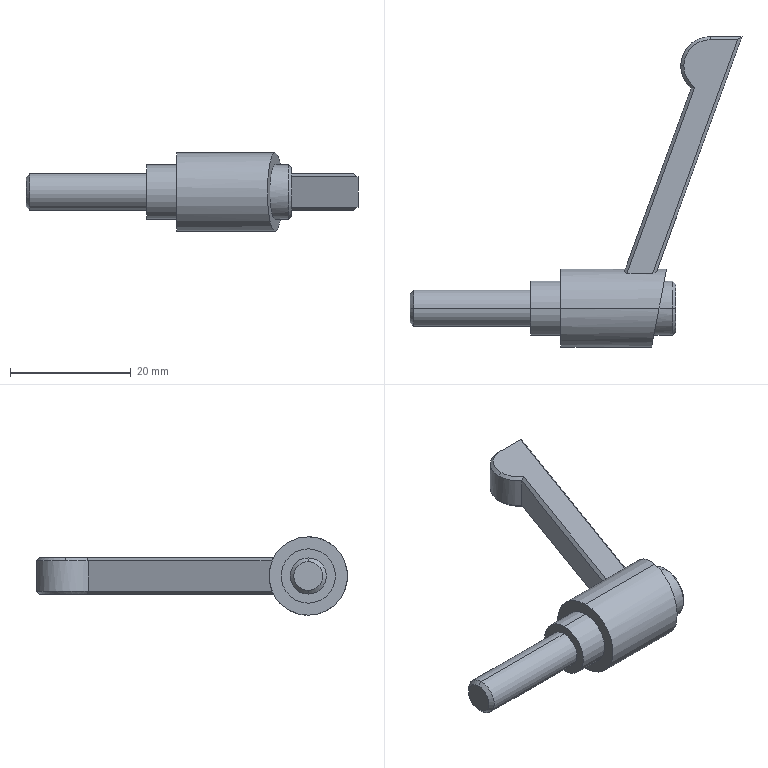Part | SolidWorks | features BaseBody 1 | 1 solid | 32 faces | box 55 x 51.5 x 13 mm | volume 4548 mm3 | plane 16 | cylinder 9 | cone 7 | commonest cylinder face diameters 9 x4 6 x2 13 x2 9.696 x1
STEP:
#1=CARTESIAN_POINT('',(15.931,5.766,-3.));
#2=VERTEX_POINT('',#1);
#3=CARTESIAN_POINT('',(20.188,5.766,-3.));
#4=VERTEX_POINT('',#3);
#5=CARTESIAN_POINT('',(25.5,5.766,-3.));
#6=DIRECTION('',(1.,0.,0.));
#7=VECTOR('',#6,1000.);
#8=LINE('',#5,#7);
#9=EDGE_CURVE('',#2,#4,#8,.T.);
#10=ORIENTED_EDGE('',*,*,#9,.T.);
#11=CARTESIAN_POINT('',(20.805,6.,-2.5));
#12=VERTEX_POINT('',#11);
#13=CARTESIAN_POINT('',(20.188,5.766,-3.));
#14=CARTESIAN_POINT('',(20.393,5.851,-2.837));
#15=CARTESIAN_POINT('',(20.599,5.929,-2.67));
#16=CARTESIAN_POINT('',(20.805,6.,-2.5));
#17=(BOUNDED_CURVE()B_SPLINE_CURVE(3,(#13,#14,#15,#16),.UNSPECIFIED.,.F.,.F.)B_SPLINE_CURVE_WITH_KNOTS((4,4),(4.562,4.647),.UNSPECIFIED.)CURVE()GEOMETRIC_REPRESENTATION_ITEM()RATIONAL_B_SPLINE_CURVE((1.,0.9994,0.9994,1.))REPRESENTATION_ITEM(''));
#18=EDGE_CURVE('',#4,#12,#17,.T.);
#19=ORIENTED_EDGE('',*,*,#18,.T.);
#20=CARTESIAN_POINT('',(20.805,6.,2.5));
#21=VERTEX_POINT('',#20);
#22=CARTESIAN_POINT('',(20.805,6.,-2.5));
#23=CARTESIAN_POINT('',(21.051,6.676,-0.8784));
#24=CARTESIAN_POINT('',(21.051,6.676,0.8784));
#25=CARTESIAN_POINT('',(20.805,6.,2.5));
#26=(BOUNDED_CURVE()B_SPLINE_CURVE(3,(#22,#23,#24,#25),.UNSPECIFIED.,.F.,.F.)B_SPLINE_CURVE_WITH_KNOTS((4,4),(5.888,6.678),.UNSPECIFIED.)CURVE()GEOMETRIC_REPRESENTATION_ITEM()RATIONAL_B_SPLINE_CURVE((1.,0.9487,0.9487,1.))REPRESENTATION_ITEM(''));
#27=EDGE_CURVE('',#12,#21,#26,.T.);
#28=ORIENTED_EDGE('',*,*,#27,.T.);
#29=CARTESIAN_POINT('',(20.188,5.766,3.));
#30=VERTEX_POINT('',#29);
#31=CARTESIAN_POINT('',(20.188,5.766,3.));
#32=CARTESIAN_POINT('',(20.393,5.851,2.837));
#33=CARTESIAN_POINT('',(20.599,5.929,2.67));
#34=CARTESIAN_POINT('',(20.805,6.,2.5));
#35=(BOUNDED_CURVE()B_SPLINE_CURVE(3,(#31,#32,#33,#34),.UNSPECIFIED.,.F.,.F.)B_SPLINE_CURVE_WITH_KNOTS((4,4),(4.562,4.647),.UNSPECIFIED.)CURVE()GEOMETRIC_REPRESENTATION_ITEM()RATIONAL_B_SPLINE_CURVE((1.,0.9994,0.9994,1.))REPRESENTATION_ITEM(''));
#36=EDGE_CURVE('',#30,#21,#35,.T.);
#37=ORIENTED_EDGE('',*,*,#36,.F.);
#38=CARTESIAN_POINT('',(15.931,5.766,3.));
#39=VERTEX_POINT('',#38);
#40=CARTESIAN_POINT('',(25.5,5.766,3.));
#41=DIRECTION('',(-1.,0.,0.));
#42=VECTOR('',#41,1000.);
#43=LINE('',#40,#42);
#44=EDGE_CURVE('',#30,#39,#43,.T.);
#45=ORIENTED_EDGE('',*,*,#44,.T.);
#46=CARTESIAN_POINT('',(15.484,6.,2.5));
#47=VERTEX_POINT('',#46);
#48=CARTESIAN_POINT('',(15.484,6.,2.5));
#49=CARTESIAN_POINT('',(15.639,5.929,2.67));
#50=CARTESIAN_POINT('',(15.788,5.851,2.837));
#51=CARTESIAN_POINT('',(15.931,5.766,3.));
#52=(BOUNDED_CURVE()B_SPLINE_CURVE(3,(#48,#49,#50,#51),.UNSPECIFIED.,.F.,.F.)B_SPLINE_CURVE_WITH_KNOTS((4,4),(5.437,5.522),.UNSPECIFIED.)CURVE()GEOMETRIC_REPRESENTATION_ITEM()RATIONAL_B_SPLINE_CURVE((1.,0.9994,0.9994,1.))REPRESENTATION_ITEM(''));
#53=EDGE_CURVE('',#47,#39,#52,.T.);
#54=ORIENTED_EDGE('',*,*,#53,.F.);
#55=CARTESIAN_POINT('',(15.484,6.,-2.5));
#56=VERTEX_POINT('',#55);
#57=CARTESIAN_POINT('',(15.484,6.,2.5));
#58=CARTESIAN_POINT('',(15.73,6.676,0.8784));
#59=CARTESIAN_POINT('',(15.73,6.676,-0.8784));
#60=CARTESIAN_POINT('',(15.484,6.,-2.5));
#61=(BOUNDED_CURVE()B_SPLINE_CURVE(3,(#57,#58,#59,#60),.UNSPECIFIED.,.F.,.F.)B_SPLINE_CURVE_WITH_KNOTS((4,4),(5.888,6.678),.UNSPECIFIED.)CURVE()GEOMETRIC_REPRESENTATION_ITEM()RATIONAL_B_SPLINE_CURVE((1.,0.9487,0.9487,1.))REPRESENTATION_ITEM(''));
#62=EDGE_CURVE('',#47,#56,#61,.T.);
#63=ORIENTED_EDGE('',*,*,#62,.T.);
#64=CARTESIAN_POINT('',(15.484,6.,-2.5));
#65=CARTESIAN_POINT('',(15.639,5.929,-2.67));
#66=CARTESIAN_POINT('',(15.788,5.851,-2.837));
#67=CARTESIAN_POINT('',(15.931,5.766,-3.));
#68=(BOUNDED_CURVE()B_SPLINE_CURVE(3,(#64,#65,#66,#67),.UNSPECIFIED.,.F.,.T.)B_SPLINE_CURVE_WITH_KNOTS((4,4),(5.437,5.522),.UNSPECIFIED.)CURVE()GEOMETRIC_REPRESENTATION_ITEM()RATIONAL_B_SPLINE_CURVE((1.,0.9994,0.9994,1.))REPRESENTATION_ITEM(''));
#69=EDGE_CURVE('',#56,#2,#68,.T.);
#70=ORIENTED_EDGE('',*,*,#69,.T.);
#71=EDGE_LOOP('',(#10,#19,#28,#37,#45,#54,#63,#70));
#72=FACE_BOUND('',#71,.T.);
#73=CARTESIAN_POINT('',(5.,0.,-6.5));
#74=VERTEX_POINT('',#73);
#75=CARTESIAN_POINT('',(5.,0.,6.5));
#76=VERTEX_POINT('',#75);
#77=CARTESIAN_POINT('',(5.,0.,0.));
#78=DIRECTION('',(1.,0.,0.));
#79=DIRECTION('',(0.,0.,-1.));
#80=AXIS2_PLACEMENT_3D('',#77,#78,#79);
#81=CIRCLE('',#80,6.5);
#82=EDGE_CURVE('',#74,#76,#81,.T.);
#83=ORIENTED_EDGE('',*,*,#82,.T.);
#84=CARTESIAN_POINT('',(21.25,0.,6.5));
#85=VERTEX_POINT('',#84);
#86=CARTESIAN_POINT('',(25.5,0.,6.5));
#87=DIRECTION('',(1.,0.,0.));
#88=VECTOR('',#87,1000.);
#89=LINE('',#86,#88);
#90=EDGE_CURVE('',#76,#85,#89,.T.);
#91=ORIENTED_EDGE('',*,*,#90,.T.);
#92=CARTESIAN_POINT('',(21.25,0.,-6.5));
#93=VERTEX_POINT('',#92);
#94=CARTESIAN_POINT('',(21.25,0.,6.5));
#95=CARTESIAN_POINT('',(23.75,13.,6.5));
#96=CARTESIAN_POINT('',(23.75,13.,-6.5));
#97=CARTESIAN_POINT('',(21.25,0.,-6.5));
#98=(BOUNDED_CURVE()B_SPLINE_CURVE(3,(#94,#95,#96,#97),.UNSPECIFIED.,.F.,.F.)B_SPLINE_CURVE_WITH_KNOTS((4,4),(4.712,7.854),.UNSPECIFIED.)CURVE()GEOMETRIC_REPRESENTATION_ITEM()RATIONAL_B_SPLINE_CURVE((1.,0.3333,0.3333,1.))REPRESENTATION_ITEM(''));
#99=EDGE_CURVE('',#85,#93,#98,.T.);
#100=ORIENTED_EDGE('',*,*,#99,.T.);
#101=CARTESIAN_POINT('',(25.5,0.,-6.5));
#102=DIRECTION('',(1.,0.,0.));
#103=VECTOR('',#102,1000.);
#104=LINE('',#101,#103);
#105=EDGE_CURVE('',#74,#93,#104,.T.);
#106=ORIENTED_EDGE('',*,*,#105,.F.);
#107=EDGE_LOOP('',(#83,#91,#100,#106));
#108=FACE_OUTER_BOUND('',#107,.T.);
#109=CARTESIAN_POINT('',(25.5,0.,0.));
#110=DIRECTION('',(1.,0.,0.));
#111=DIRECTION('',(0.,0.,-1.));
#112=AXIS2_PLACEMENT_3D('',#109,#110,#111);
#113=CYLINDRICAL_SURFACE('',#112,6.5);
#114=ADVANCED_FACE('',(#72,#108),#113,.T.);
#115=CARTESIAN_POINT('',(21.25,0.,4.5));
#116=VERTEX_POINT('',#115);
#117=CARTESIAN_POINT('',(21.25,0.,-4.5));
#118=VERTEX_POINT('',#117);
#119=CARTESIAN_POINT('',(21.25,0.,4.5));
#120=CARTESIAN_POINT('',(22.981,9.,4.5));
#121=CARTESIAN_POINT('',(22.981,9.,-4.5));
#122=CARTESIAN_POINT('',(21.25,0.,-4.5));
#123=(BOUNDED_CURVE()B_SPLINE_CURVE(3,(#119,#120,#121,#122),.UNSPECIFIED.,.F.,.F.)B_SPLINE_CURVE_WITH_KNOTS((4,4),(4.712,7.854),.UNSPECIFIED.)CURVE()GEOMETRIC_REPRESENTATION_ITEM()RATIONAL_B_SPLINE_CURVE((1.,0.3333,0.3333,1.))REPRESENTATION_ITEM(''));
#124=EDGE_CURVE('',#116,#118,#123,.T.);
#125=ORIENTED_EDGE('',*,*,#124,.F.);
#126=CARTESIAN_POINT('',(23.5,0.,4.5));
#127=VERTEX_POINT('',#126);
#128=CARTESIAN_POINT('',(24.,0.,4.5));
#129=DIRECTION('',(1.,0.,0.));
#130=VECTOR('',#129,1000.);
#131=LINE('',#128,#130);
#132=EDGE_CURVE('',#116,#127,#131,.T.);
#133=ORIENTED_EDGE('',*,*,#132,.T.);
#134=CARTESIAN_POINT('',(23.5,0.,-4.5));
#135=VERTEX_POINT('',#134);
#136=CARTESIAN_POINT('',(23.5,0.,0.));
#137=DIRECTION('',(-1.,0.,0.));
#138=DIRECTION('',(0.,0.,-1.));
#139=AXIS2_PLACEMENT_3D('',#136,#137,#138);
#140=CIRCLE('',#139,4.5);
#141=EDGE_CURVE('',#127,#135,#140,.T.);
#142=ORIENTED_EDGE('',*,*,#141,.T.);
#143=CARTESIAN_POINT('',(24.,0.,-4.5));
#144=DIRECTION('',(1.,0.,0.));
#145=VECTOR('',#144,1000.);
#146=LINE('',#143,#145);
#147=EDGE_CURVE('',#118,#135,#146,.T.);
#148=ORIENTED_EDGE('',*,*,#147,.F.);
#149=EDGE_LOOP('',(#125,#133,#142,#148));
#150=FACE_OUTER_BOUND('',#149,.T.);
#151=CARTESIAN_POINT('',(24.,0.,0.));
#152=DIRECTION('',(1.,0.,0.));
#153=DIRECTION('',(0.,0.,-1.));
#154=AXIS2_PLACEMENT_3D('',#151,#152,#153);
#155=CYLINDRICAL_SURFACE('',#154,4.5);
#156=ADVANCED_FACE('',(#150),#155,.T.);
#157=CARTESIAN_POINT('',(25.364,40.152,3.));
#158=VERTEX_POINT('',#157);
#159=CARTESIAN_POINT('',(27.164,36.629,3.));
#160=VERTEX_POINT('',#159);
#161=CARTESIAN_POINT('',(29.712,40.152,3.));
#162=DIRECTION('',(0.,0.,1.));
#163=DIRECTION('',(-1.,0.,0.));
#164=AXIS2_PLACEMENT_3D('',#161,#162,#163);
#165=CIRCLE('',#164,4.348);
#166=EDGE_CURVE('',#158,#160,#165,.T.);
#167=ORIENTED_EDGE('',*,*,#166,.F.);
#168=CARTESIAN_POINT('',(24.864,40.152,2.5));
#169=VERTEX_POINT('',#168);
#170=CARTESIAN_POINT('',(24.864,40.152,2.5));
#171=DIRECTION('',(-0.7071,0.,-0.7071));
#172=VECTOR('',#171,1000.);
#173=LINE('',#170,#172);
#174=EDGE_CURVE('',#158,#169,#173,.T.);
#175=ORIENTED_EDGE('',*,*,#174,.T.);
#176=CARTESIAN_POINT('',(26.571,36.46,2.5));
#177=VERTEX_POINT('',#176);
#178=CARTESIAN_POINT('',(29.712,40.152,2.5));
#179=DIRECTION('',(0.,0.,-1.));
#180=DIRECTION('',(1.,0.,0.));
#181=AXIS2_PLACEMENT_3D('',#178,#179,#180);
#182=CIRCLE('',#181,4.848);
#183=EDGE_CURVE('',#177,#169,#182,.T.);
#184=ORIENTED_EDGE('',*,*,#183,.F.);
#185=CARTESIAN_POINT('',(27.164,36.629,3.));
#186=CARTESIAN_POINT('',(26.966,36.568,2.835));
#187=CARTESIAN_POINT('',(26.769,36.512,2.668));
#188=CARTESIAN_POINT('',(26.571,36.46,2.5));
#189=B_SPLINE_CURVE_WITH_KNOTS('',3,(#185,#186,#187,#188),.UNSPECIFIED.,.F.,.F.,(4,4),(0.,0.0007944),.UNSPECIFIED.);
#190=EDGE_CURVE('',#160,#177,#189,.T.);
#191=ORIENTED_EDGE('',*,*,#190,.F.);
#192=EDGE_LOOP('',(#167,#175,#184,#191));
#193=FACE_OUTER_BOUND('',#192,.T.);
#194=CARTESIAN_POINT('',(29.712,40.152,2.5));
#195=DIRECTION('',(0.,0.,-1.));
#196=DIRECTION('',(-1.,0.,0.));
#197=AXIS2_PLACEMENT_3D('',#194,#195,#196);
#198=CONICAL_SURFACE('',#197,4.848,0.7854);
#199=ADVANCED_FACE('',(#193),#198,.T.);
#200=CARTESIAN_POINT('',(0.,0.,-4.5));
#201=VERTEX_POINT('',#200);
#202=CARTESIAN_POINT('',(0.,0.,4.5));
#203=VERTEX_POINT('',#202);
#204=CARTESIAN_POINT('',(0.,0.,0.));
#205=DIRECTION('',(1.,0.,0.));
#206=DIRECTION('',(0.,0.,-1.));
#207=AXIS2_PLACEMENT_3D('',#204,#205,#206);
#208=CIRCLE('',#207,4.5);
#209=EDGE_CURVE('',#201,#203,#208,.T.);
#210=ORIENTED_EDGE('',*,*,#209,.T.);
#211=CARTESIAN_POINT('',(5.,0.,4.5));
#212=VERTEX_POINT('',#211);
#213=CARTESIAN_POINT('',(24.,0.,4.5));
#214=DIRECTION('',(1.,0.,0.));
#215=VECTOR('',#214,1000.);
#216=LINE('',#213,#215);
#217=EDGE_CURVE('',#203,#212,#216,.T.);
#218=ORIENTED_EDGE('',*,*,#217,.T.);
#219=CARTESIAN_POINT('',(5.,0.,-4.5));
#220=VERTEX_POINT('',#219);
#221=CARTESIAN_POINT('',(5.,0.,0.));
#222=DIRECTION('',(1.,0.,0.));
#223=DIRECTION('',(0.,0.,-1.));
#224=AXIS2_PLACEMENT_3D('',#221,#222,#223);
#225=CIRCLE('',#224,4.5);
#226=EDGE_CURVE('',#220,#212,#225,.T.);
#227=ORIENTED_EDGE('',*,*,#226,.F.);
#228=CARTESIAN_POINT('',(24.,0.,-4.5));
#229=DIRECTION('',(1.,0.,0.));
#230=VECTOR('',#229,1000.);
#231=LINE('',#228,#230);
#232=EDGE_CURVE('',#201,#220,#231,.T.);
#233=ORIENTED_EDGE('',*,*,#232,.F.);
#234=EDGE_LOOP('',(#210,#218,#227,#233));
#235=FACE_OUTER_BOUND('',#234,.T.);
#236=CARTESIAN_POINT('',(24.,0.,0.));
#237=DIRECTION('',(1.,0.,0.));
#238=DIRECTION('',(0.,0.,-1.));
#239=AXIS2_PLACEMENT_3D('',#236,#237,#238);
#240=CYLINDRICAL_SURFACE('',#239,4.5);
#241=ADVANCED_FACE('',(#235),#240,.T.);
#242=CARTESIAN_POINT('',(24.,0.,4.));
#243=VERTEX_POINT('',#242);
#244=CARTESIAN_POINT('',(24.,0.,-4.));
#245=VERTEX_POINT('',#244);
#246=CARTESIAN_POINT('',(24.,0.,0.));
#247=DIRECTION('',(-1.,0.,0.));
#248=DIRECTION('',(0.,0.,1.));
#249=AXIS2_PLACEMENT_3D('',#246,#247,#248);
#250=CIRCLE('',#249,4.);
#251=EDGE_CURVE('',#243,#245,#250,.T.);
#252=ORIENTED_EDGE('',*,*,#251,.T.);
#253=CARTESIAN_POINT('',(23.5,0.,-4.5));
#254=DIRECTION('',(-0.7071,0.,-0.7071));
#255=VECTOR('',#254,1000.);
#256=LINE('',#253,#255);
#257=EDGE_CURVE('',#245,#135,#256,.T.);
#258=ORIENTED_EDGE('',*,*,#257,.T.);
#259=ORIENTED_EDGE('',*,*,#141,.F.);
#260=CARTESIAN_POINT('',(23.5,0.,4.5));
#261=DIRECTION('',(-0.7071,0.,0.7071));
#262=VECTOR('',#261,1000.);
#263=LINE('',#260,#262);
#264=EDGE_CURVE('',#243,#127,#263,.T.);
#265=ORIENTED_EDGE('',*,*,#264,.F.);
#266=EDGE_LOOP('',(#252,#258,#259,#265));
#267=FACE_OUTER_BOUND('',#266,.T.);
#268=CARTESIAN_POINT('',(23.5,0.,0.));
#269=DIRECTION('',(-1.,0.,0.));
#270=DIRECTION('',(0.,0.,1.));
#271=AXIS2_PLACEMENT_3D('',#268,#269,#270);
#272=CONICAL_SURFACE('',#271,4.5,0.7854);
#273=ADVANCED_FACE('',(#267),#272,.T.);
#274=CARTESIAN_POINT('',(0.,0.,3.));
#275=VERTEX_POINT('',#274);
#276=CARTESIAN_POINT('',(0.,0.,-3.));
#277=VERTEX_POINT('',#276);
#278=CARTESIAN_POINT('',(0.,0.,0.));
#279=DIRECTION('',(-1.,0.,0.));
#280=DIRECTION('',(0.,0.,1.));
#281=AXIS2_PLACEMENT_3D('',#278,#279,#280);
#282=CIRCLE('',#281,3.);
#283=EDGE_CURVE('',#275,#277,#282,.T.);
#284=ORIENTED_EDGE('',*,*,#283,.T.);
#285=CARTESIAN_POINT('',(-19.387,0.,-3.));
#286=VERTEX_POINT('',#285);
#287=CARTESIAN_POINT('',(0.,0.,-3.));
#288=DIRECTION('',(-1.,0.,0.));
#289=VECTOR('',#288,1000.);
#290=LINE('',#287,#289);
#291=EDGE_CURVE('',#277,#286,#290,.T.);
#292=ORIENTED_EDGE('',*,*,#291,.T.);
#293=CARTESIAN_POINT('',(-19.387,0.,3.));
#294=VERTEX_POINT('',#293);
#295=CARTESIAN_POINT('',(-19.387,0.,0.));
#296=DIRECTION('',(1.,0.,0.));
#297=DIRECTION('',(0.,0.,1.));
#298=AXIS2_PLACEMENT_3D('',#295,#296,#297);
#299=CIRCLE('',#298,3.);
#300=EDGE_CURVE('',#286,#294,#299,.T.);
#301=ORIENTED_EDGE('',*,*,#300,.T.);
#302=CARTESIAN_POINT('',(0.,0.,3.));
#303=DIRECTION('',(-1.,0.,0.));
#304=VECTOR('',#303,1000.);
#305=LINE('',#302,#304);
#306=EDGE_CURVE('',#275,#294,#305,.T.);
#307=ORIENTED_EDGE('',*,*,#306,.F.);
#308=EDGE_LOOP('',(#284,#292,#301,#307));
#309=FACE_OUTER_BOUND('',#308,.T.);
#310=CARTESIAN_POINT('',(0.,0.,0.));
#311=DIRECTION('',(-1.,0.,0.));
#312=DIRECTION('',(0.,0.,1.));
#313=AXIS2_PLACEMENT_3D('',#310,#311,#312);
#314=CYLINDRICAL_SURFACE('',#313,3.);
#315=ADVANCED_FACE('',(#309),#314,.T.);
#316=CARTESIAN_POINT('',(-20.,0.,-2.387));
#317=VERTEX_POINT('',#316);
#318=CARTESIAN_POINT('',(-20.,0.,2.387));
#319=VERTEX_POINT('',#318);
#320=CARTESIAN_POINT('',(-20.,0.,0.));
#321=DIRECTION('',(1.,0.,0.));
#322=DIRECTION('',(0.,0.,-1.));
#323=AXIS2_PLACEMENT_3D('',#320,#321,#322);
#324=CIRCLE('',#323,2.387);
#325=EDGE_CURVE('',#317,#319,#324,.T.);
#326=ORIENTED_EDGE('',*,*,#325,.T.);
#327=CARTESIAN_POINT('',(-19.386,0.,3.));
#328=DIRECTION('',(0.7071,0.,0.7071));
#329=VECTOR('',#328,1000.);
#330=LINE('',#327,#329);
#331=EDGE_CURVE('',#319,#294,#330,.T.);
#332=ORIENTED_EDGE('',*,*,#331,.T.);
#333=ORIENTED_EDGE('',*,*,#300,.F.);
#334=CARTESIAN_POINT('',(-19.386,0.,-3.));
#335=DIRECTION('',(0.7071,0.,-0.7071));
#336=VECTOR('',#335,1000.);
#337=LINE('',#334,#336);
#338=EDGE_CURVE('',#317,#286,#337,.T.);
#339=ORIENTED_EDGE('',*,*,#338,.F.);
#340=EDGE_LOOP('',(#326,#332,#333,#339));
#341=FACE_OUTER_BOUND('',#340,.T.);
#342=CARTESIAN_POINT('',(-19.386,0.,0.));
#343=DIRECTION('',(1.,0.,0.));
#344=DIRECTION('',(0.,0.,-1.));
#345=AXIS2_PLACEMENT_3D('',#342,#343,#344);
#346=CONICAL_SURFACE('',#345,3.,0.7854);
#347=ADVANCED_FACE('',(#341),#346,.T.);
#348=ORIENTED_EDGE('',*,*,#90,.F.);
#349=CARTESIAN_POINT('',(5.,0.,0.));
#350=DIRECTION('',(1.,0.,0.));
#351=DIRECTION('',(0.,0.,-1.));
#352=AXIS2_PLACEMENT_3D('',#349,#350,#351);
#353=CIRCLE('',#352,6.5);
#354=EDGE_CURVE('',#76,#74,#353,.T.);
#355=ORIENTED_EDGE('',*,*,#354,.T.);
#356=ORIENTED_EDGE('',*,*,#105,.T.);
#357=CARTESIAN_POINT('',(21.25,0.,-6.5));
#358=CARTESIAN_POINT('',(18.75,-13.,-6.5));
#359=CARTESIAN_POINT('',(18.75,-13.,6.5));
#360=CARTESIAN_POINT('',(21.25,0.,6.5));
#361=(BOUNDED_CURVE()B_SPLINE_CURVE(3,(#357,#358,#359,#360),.UNSPECIFIED.,.F.,.F.)B_SPLINE_CURVE_WITH_KNOTS((4,4),(1.571,4.712),.UNSPECIFIED.)CURVE()GEOMETRIC_REPRESENTATION_ITEM()RATIONAL_B_SPLINE_CURVE((1.,0.3333,0.3333,1.))REPRESENTATION_ITEM(''));
#362=EDGE_CURVE('',#93,#85,#361,.T.);
#363=ORIENTED_EDGE('',*,*,#362,.T.);
#364=EDGE_LOOP('',(#348,#355,#356,#363));
#365=FACE_OUTER_BOUND('',#364,.T.);
#366=CARTESIAN_POINT('',(25.5,0.,0.));
#367=DIRECTION('',(1.,0.,0.));
#368=DIRECTION('',(0.,0.,-1.));
#369=AXIS2_PLACEMENT_3D('',#366,#367,#368);
#370=CYLINDRICAL_SURFACE('',#369,6.5);
#371=ADVANCED_FACE('',(#365),#370,.T.);
#372=ORIENTED_EDGE('',*,*,#362,.F.);
#373=ORIENTED_EDGE('',*,*,#99,.F.);
#374=EDGE_LOOP('',(#372,#373));
#375=FACE_OUTER_BOUND('',#374,.T.);
#376=CARTESIAN_POINT('',(21.25,0.,-4.5));
#377=CARTESIAN_POINT('',(19.519,-9.,-4.5));
#378=CARTESIAN_POINT('',(19.519,-9.,4.5));
#379=CARTESIAN_POINT('',(21.25,0.,4.5));
#380=(BOUNDED_CURVE()B_SPLINE_CURVE(3,(#376,#377,#378,#379),.UNSPECIFIED.,.F.,.F.)B_SPLINE_CURVE_WITH_KNOTS((4,4),(1.571,4.712),.UNSPECIFIED.)CURVE()GEOMETRIC_REPRESENTATION_ITEM()RATIONAL_B_SPLINE_CURVE((1.,0.3333,0.3333,1.))REPRESENTATION_ITEM(''));
#381=EDGE_CURVE('',#118,#116,#380,.T.);
#382=ORIENTED_EDGE('',*,*,#381,.T.);
#383=ORIENTED_EDGE('',*,*,#124,.T.);
#384=EDGE_LOOP('',(#382,#383));
#385=FACE_BOUND('',#384,.T.);
#386=CARTESIAN_POINT('',(22.5,6.5,6.5));
#387=DIRECTION('',(0.982,-0.1888,0.));
#388=DIRECTION('',(0.1888,0.982,0.));
#389=AXIS2_PLACEMENT_3D('',#386,#387,#388);
#390=PLANE('',#389);
#391=ADVANCED_FACE('',(#375,#385),#390,.T.);
#392=CARTESIAN_POINT('',(34.286,44.5,-3.));
#393=VERTEX_POINT('',#392);
#394=CARTESIAN_POINT('',(20.188,5.766,-3.));
#395=DIRECTION('',(0.342,0.9397,0.));
#396=VECTOR('',#395,1000.);
#397=LINE('',#394,#396);
#398=EDGE_CURVE('',#4,#393,#397,.T.);
#399=ORIENTED_EDGE('',*,*,#398,.F.);
#400=ORIENTED_EDGE('',*,*,#9,.F.);
#401=CARTESIAN_POINT('',(27.164,36.629,-3.));
#402=VERTEX_POINT('',#401);
#403=CARTESIAN_POINT('',(27.164,36.629,-3.));
#404=DIRECTION('',(-0.342,-0.9397,0.));
#405=VECTOR('',#404,1000.);
#406=LINE('',#403,#405);
#407=EDGE_CURVE('',#402,#2,#406,.T.);
#408=ORIENTED_EDGE('',*,*,#407,.F.);
#409=CARTESIAN_POINT('',(29.744,44.5,-3.));
#410=VERTEX_POINT('',#409);
#411=CARTESIAN_POINT('',(29.712,40.152,-3.));
#412=DIRECTION('',(0.,0.,1.));
#413=DIRECTION('',(1.,0.,0.));
#414=AXIS2_PLACEMENT_3D('',#411,#412,#413);
#415=CIRCLE('',#414,4.348);
#416=EDGE_CURVE('',#410,#402,#415,.T.);
#417=ORIENTED_EDGE('',*,*,#416,.F.);
#418=CARTESIAN_POINT('',(29.712,44.5,-3.));
#419=DIRECTION('',(-1.,0.,0.));
#420=VECTOR('',#419,1000.);
#421=LINE('',#418,#420);
#422=EDGE_CURVE('',#393,#410,#421,.T.);
#423=ORIENTED_EDGE('',*,*,#422,.F.);
#424=EDGE_LOOP('',(#399,#400,#408,#417,#423));
#425=FACE_OUTER_BOUND('',#424,.T.);
#426=CARTESIAN_POINT('',(29.712,40.152,-3.));
#427=DIRECTION('',(0.,0.,1.));
#428=DIRECTION('',(1.,0.,0.));
#429=AXIS2_PLACEMENT_3D('',#426,#427,#428);
#430=PLANE('',#429);
#431=ADVANCED_FACE('',(#425),#430,.F.);
#432=CARTESIAN_POINT('',(26.571,36.46,2.5));
#433=DIRECTION('',(-0.342,-0.9397,0.));
#434=VECTOR('',#433,1000.);
#435=LINE('',#432,#434);
#436=EDGE_CURVE('',#177,#47,#435,.T.);
#437=ORIENTED_EDGE('',*,*,#436,.F.);
#438=CARTESIAN_POINT('',(26.571,36.46,-2.5));
#439=VERTEX_POINT('',#438);
#440=CARTESIAN_POINT('',(26.571,36.46,3.));
#441=DIRECTION('',(0.,0.,1.));
#442=VECTOR('',#441,1000.);
#443=LINE('',#440,#442);
#444=EDGE_CURVE('',#439,#177,#443,.T.);
#445=ORIENTED_EDGE('',*,*,#444,.F.);
#446=CARTESIAN_POINT('',(26.571,36.46,-2.5));
#447=DIRECTION('',(0.342,0.9397,0.));
#448=VECTOR('',#447,1000.);
#449=LINE('',#446,#448);
#450=EDGE_CURVE('',#56,#439,#449,.T.);
#451=ORIENTED_EDGE('',*,*,#450,.F.);
#452=ORIENTED_EDGE('',*,*,#62,.F.);
#453=EDGE_LOOP('',(#437,#445,#451,#452));
#454=FACE_OUTER_BOUND('',#453,.T.);
#455=CARTESIAN_POINT('',(26.571,36.46,3.));
#456=DIRECTION('',(0.9397,-0.342,0.));
#457=DIRECTION('',(0.342,0.9397,0.));
#458=AXIS2_PLACEMENT_3D('',#455,#456,#457);
#459=PLANE('',#458);
#460=ADVANCED_FACE('',(#454),#459,.F.);
#461=CARTESIAN_POINT('',(34.286,44.5,3.));
#462=VERTEX_POINT('',#461);
#463=CARTESIAN_POINT('',(20.188,5.766,3.));
#464=DIRECTION('',(0.342,0.9397,0.));
#465=VECTOR('',#464,1000.);
#466=LINE('',#463,#465);
#467=EDGE_CURVE('',#30,#462,#466,.T.);
#468=ORIENTED_EDGE('',*,*,#467,.T.);
#469=CARTESIAN_POINT('',(29.744,44.5,3.));
#470=VERTEX_POINT('',#469);
#471=CARTESIAN_POINT('',(29.712,44.5,3.));
#472=DIRECTION('',(-1.,0.,0.));
#473=VECTOR('',#472,1000.);
#474=LINE('',#471,#473);
#475=EDGE_CURVE('',#462,#470,#474,.T.);
#476=ORIENTED_EDGE('',*,*,#475,.T.);
#477=CARTESIAN_POINT('',(29.712,40.152,3.));
#478=DIRECTION('',(0.,0.,1.));
#479=DIRECTION('',(-1.,0.,0.));
#480=AXIS2_PLACEMENT_3D('',#477,#478,#479);
#481=CIRCLE('',#480,4.348);
#482=EDGE_CURVE('',#470,#158,#481,.T.);
#483=ORIENTED_EDGE('',*,*,#482,.T.);
#484=ORIENTED_EDGE('',*,*,#166,.T.);
#485=CARTESIAN_POINT('',(27.164,36.629,3.));
#486=DIRECTION('',(-0.342,-0.9397,0.));
#487=VECTOR('',#486,1000.);
#488=LINE('',#485,#487);
#489=EDGE_CURVE('',#160,#39,#488,.T.);
#490=ORIENTED_EDGE('',*,*,#489,.T.);
#491=ORIENTED_EDGE('',*,*,#44,.F.);
#492=EDGE_LOOP('',(#468,#476,#483,#484,#490,#491));
#493=FACE_OUTER_BOUND('',#492,.T.);
#494=CARTESIAN_POINT('',(29.712,40.152,3.));
#495=DIRECTION('',(0.,0.,1.));
#496=DIRECTION('',(1.,0.,0.));
#497=AXIS2_PLACEMENT_3D('',#494,#495,#496);
#498=PLANE('',#497);
#499=ADVANCED_FACE('',(#493),#498,.T.);
#500=CARTESIAN_POINT('',(35.,45.,-2.5));
#501=VERTEX_POINT('',#500);
#502=CARTESIAN_POINT('',(18.621,0.,-2.5));
#503=DIRECTION('',(-0.342,-0.9397,0.));
#504=VECTOR('',#503,1000.);
#505=LINE('',#502,#504);
#506=EDGE_CURVE('',#501,#12,#505,.T.);
#507=ORIENTED_EDGE('',*,*,#506,.F.);
#508=CARTESIAN_POINT('',(35.,45.,2.5));
#509=VERTEX_POINT('',#508);
#510=CARTESIAN_POINT('',(35.,45.,3.));
#511=DIRECTION('',(0.,0.,-1.));
#512=VECTOR('',#511,1000.);
#513=LINE('',#510,#512);
#514=EDGE_CURVE('',#509,#501,#513,.T.);
#515=ORIENTED_EDGE('',*,*,#514,.F.);
#516=CARTESIAN_POINT('',(18.621,0.,2.5));
#517=DIRECTION('',(0.342,0.9397,0.));
#518=VECTOR('',#517,1000.);
#519=LINE('',#516,#518);
#520=EDGE_CURVE('',#21,#509,#519,.T.);
#521=ORIENTED_EDGE('',*,*,#520,.F.);
#522=ORIENTED_EDGE('',*,*,#27,.F.);
#523=EDGE_LOOP('',(#507,#515,#521,#522));
#524=FACE_OUTER_BOUND('',#523,.T.);
#525=CARTESIAN_POINT('',(18.621,0.,3.));
#526=DIRECTION('',(-0.9397,0.342,0.));
#527=DIRECTION('',(-0.342,-0.9397,0.));
#528=AXIS2_PLACEMENT_3D('',#525,#526,#527);
#529=PLANE('',#528);
#530=ADVANCED_FACE('',(#524),#529,.F.);
#531=ORIENTED_EDGE('',*,*,#82,.F.);
#532=ORIENTED_EDGE('',*,*,#354,.F.);
#533=EDGE_LOOP('',(#531,#532));
#534=FACE_OUTER_BOUND('',#533,.T.);
#535=ORIENTED_EDGE('',*,*,#226,.T.);
#536=CARTESIAN_POINT('',(5.,0.,0.));
#537=DIRECTION('',(1.,0.,0.));
#538=DIRECTION('',(0.,0.,-1.));
#539=AXIS2_PLACEMENT_3D('',#536,#537,#538);
#540=CIRCLE('',#539,4.5);
#541=EDGE_CURVE('',#212,#220,#540,.T.);
#542=ORIENTED_EDGE('',*,*,#541,.T.);
#543=EDGE_LOOP('',(#535,#542));
#544=FACE_BOUND('',#543,.T.);
#545=CARTESIAN_POINT('',(5.,-6.5,6.5));
#546=DIRECTION('',(-1.,0.,0.));
#547=DIRECTION('',(0.,0.,1.));
#548=AXIS2_PLACEMENT_3D('',#545,#546,#547);
#549=PLANE('',#548);
#550=ADVANCED_FACE('',(#534,#544),#549,.T.);
#551=ORIENTED_EDGE('',*,*,#132,.F.);
#552=ORIENTED_EDGE('',*,*,#381,.F.);
#553=ORIENTED_EDGE('',*,*,#147,.T.);
#554=CARTESIAN_POINT('',(23.5,0.,0.));
#555=DIRECTION('',(-1.,0.,0.));
#556=DIRECTION('',(0.,0.,-1.));
#557=AXIS2_PLACEMENT_3D('',#554,#555,#556);
#558=CIRCLE('',#557,4.5);
#559=EDGE_CURVE('',#135,#127,#558,.T.);
#560=ORIENTED_EDGE('',*,*,#559,.T.);
#561=EDGE_LOOP('',(#551,#552,#553,#560));
#562=FACE_OUTER_BOUND('',#561,.T.);
#563=CARTESIAN_POINT('',(24.,0.,0.));
#564=DIRECTION('',(1.,0.,0.));
#565=DIRECTION('',(0.,0.,-1.));
#566=AXIS2_PLACEMENT_3D('',#563,#564,#565);
#567=CYLINDRICAL_SURFACE('',#566,4.5);
#568=ADVANCED_FACE('',(#562),#567,.T.);
#569=CARTESIAN_POINT('',(29.746,45.,-2.5));
#570=VERTEX_POINT('',#569);
#571=CARTESIAN_POINT('',(35.,45.,-2.5));
#572=DIRECTION('',(-1.,0.,0.));
#573=VECTOR('',#572,1000.);
#574=LINE('',#571,#573);
#575=EDGE_CURVE('',#501,#570,#574,.T.);
#576=ORIENTED_EDGE('',*,*,#575,.F.);
#577=CARTESIAN_POINT('',(34.286,44.5,-3.));
#578=DIRECTION('',(0.7106,0.4975,0.4975));
#579=VECTOR('',#578,1000.);
#580=LINE('',#577,#579);
#581=EDGE_CURVE('',#393,#501,#580,.T.);
#582=ORIENTED_EDGE('',*,*,#581,.F.);
#583=ORIENTED_EDGE('',*,*,#422,.T.);
#584=CARTESIAN_POINT('',(29.746,45.,-2.5));
#585=CARTESIAN_POINT('',(29.745,44.833,-2.667));
#586=CARTESIAN_POINT('',(29.745,44.667,-2.833));
#587=CARTESIAN_POINT('',(29.744,44.5,-3.));
#588=B_SPLINE_CURVE_WITH_KNOTS('',3,(#584,#585,#586,#587),.UNSPECIFIED.,.F.,.F.,(4,4),(0.,1.),.UNSPECIFIED.);
#589=EDGE_CURVE('',#570,#410,#588,.T.);
#590=ORIENTED_EDGE('',*,*,#589,.F.);
#591=EDGE_LOOP('',(#576,#582,#583,#590));
#592=FACE_OUTER_BOUND('',#591,.T.);
#593=CARTESIAN_POINT('',(35.,45.,-2.5));
#594=DIRECTION('',(0.,-0.7071,0.7071));
#595=DIRECTION('',(0.,-0.7071,-0.7071));
#596=AXIS2_PLACEMENT_3D('',#593,#594,#595);
#597=PLANE('',#596);
#598=ADVANCED_FACE('',(#592),#597,.F.);
#599=ORIENTED_EDGE('',*,*,#398,.T.);
#600=ORIENTED_EDGE('',*,*,#581,.T.);
#601=ORIENTED_EDGE('',*,*,#506,.T.);
#602=ORIENTED_EDGE('',*,*,#18,.F.);
#603=EDGE_LOOP('',(#599,#600,#601,#602));
#604=FACE_OUTER_BOUND('',#603,.T.);
#605=CARTESIAN_POINT('',(18.621,0.,-2.5));
#606=DIRECTION('',(-0.6645,0.2418,0.7071));
#607=DIRECTION('',(0.7287,0.,0.6848));
#608=AXIS2_PLACEMENT_3D('',#605,#606,#607);
#609=PLANE('',#608);
#610=ADVANCED_FACE('',(#604),#609,.F.);
#611=ORIENTED_EDGE('',*,*,#450,.T.);
#612=CARTESIAN_POINT('',(27.164,36.629,-3.));
#613=CARTESIAN_POINT('',(26.966,36.568,-2.835));
#614=CARTESIAN_POINT('',(26.769,36.512,-2.668));
#615=CARTESIAN_POINT('',(26.571,36.46,-2.5));
#616=B_SPLINE_CURVE_WITH_KNOTS('',3,(#612,#613,#614,#615),.UNSPECIFIED.,.F.,.F.,(4,4),(0.,0.0007944),.UNSPECIFIED.);
#617=EDGE_CURVE('',#402,#439,#616,.T.);
#618=ORIENTED_EDGE('',*,*,#617,.F.);
#619=ORIENTED_EDGE('',*,*,#407,.T.);
#620=ORIENTED_EDGE('',*,*,#69,.F.);
#621=EDGE_LOOP('',(#611,#618,#619,#620));
#622=FACE_OUTER_BOUND('',#621,.T.);
#623=CARTESIAN_POINT('',(26.571,36.46,-2.5));
#624=DIRECTION('',(0.6645,-0.2418,0.7071));
#625=DIRECTION('',(0.7287,0.,-0.6848));
#626=AXIS2_PLACEMENT_3D('',#623,#624,#625);
#627=PLANE('',#626);
#628=ADVANCED_FACE('',(#622),#627,.F.);
#629=ORIENTED_EDGE('',*,*,#589,.T.);
#630=ORIENTED_EDGE('',*,*,#416,.T.);
#631=ORIENTED_EDGE('',*,*,#617,.T.);
#632=CARTESIAN_POINT('',(29.712,40.152,-2.5));
#633=DIRECTION('',(0.,0.,-1.));
#634=DIRECTION('',(1.,0.,0.));
#635=AXIS2_PLACEMENT_3D('',#632,#633,#634);
#636=CIRCLE('',#635,4.848);
#637=EDGE_CURVE('',#439,#570,#636,.T.);
#638=ORIENTED_EDGE('',*,*,#637,.T.);
#639=EDGE_LOOP('',(#629,#630,#631,#638));
#640=FACE_OUTER_BOUND('',#639,.T.);
#641=CARTESIAN_POINT('',(29.712,40.152,-2.5));
#642=DIRECTION('',(0.,0.,1.));
#643=DIRECTION('',(1.,0.,0.));
#644=AXIS2_PLACEMENT_3D('',#641,#642,#643);
#645=CONICAL_SURFACE('',#644,4.848,0.7854);
#646=ADVANCED_FACE('',(#640),#645,.T.);
#647=ORIENTED_EDGE('',*,*,#190,.T.);
#648=ORIENTED_EDGE('',*,*,#436,.T.);
#649=ORIENTED_EDGE('',*,*,#53,.T.);
#650=ORIENTED_EDGE('',*,*,#489,.F.);
#651=EDGE_LOOP('',(#647,#648,#649,#650));
#652=FACE_OUTER_BOUND('',#651,.T.);
#653=CARTESIAN_POINT('',(28.595,40.559,3.));
#654=DIRECTION('',(-0.6645,0.2418,0.7071));
#655=DIRECTION('',(0.7287,0.,0.6848));
#656=AXIS2_PLACEMENT_3D('',#653,#654,#655);
#657=PLANE('',#656);
#658=ADVANCED_FACE('',(#652),#657,.T.);
#659=CARTESIAN_POINT('',(29.746,45.,2.5));
#660=VERTEX_POINT('',#659);
#661=CARTESIAN_POINT('',(29.746,45.,3.));
#662=DIRECTION('',(0.,0.,-1.));
#663=VECTOR('',#662,1000.);
#664=LINE('',#661,#663);
#665=EDGE_CURVE('',#660,#570,#664,.T.);
#666=ORIENTED_EDGE('',*,*,#665,.T.);
#667=ORIENTED_EDGE('',*,*,#637,.F.);
#668=ORIENTED_EDGE('',*,*,#444,.T.);
#669=ORIENTED_EDGE('',*,*,#183,.T.);
#670=CARTESIAN_POINT('',(29.712,40.152,2.5));
#671=DIRECTION('',(0.,0.,-1.));
#672=DIRECTION('',(1.,0.,0.));
#673=AXIS2_PLACEMENT_3D('',#670,#671,#672);
#674=CIRCLE('',#673,4.848);
#675=EDGE_CURVE('',#169,#660,#674,.T.);
#676=ORIENTED_EDGE('',*,*,#675,.T.);
#677=EDGE_LOOP('',(#666,#667,#668,#669,#676));
#678=FACE_OUTER_BOUND('',#677,.T.);
#679=CARTESIAN_POINT('',(29.712,40.152,3.));
#680=DIRECTION('',(0.,0.,1.));
#681=DIRECTION('',(1.,0.,0.));
#682=AXIS2_PLACEMENT_3D('',#679,#680,#681);
#683=CYLINDRICAL_SURFACE('',#682,4.848);
#684=ADVANCED_FACE('',(#678),#683,.T.);
#685=CARTESIAN_POINT('',(29.746,45.,2.5));
#686=DIRECTION('',(-0.002499,-0.7071,0.7071));
#687=VECTOR('',#686,1000.);
#688=LINE('',#685,#687);
#689=EDGE_CURVE('',#660,#470,#688,.T.);
#690=ORIENTED_EDGE('',*,*,#689,.T.);
#691=ORIENTED_EDGE('',*,*,#475,.F.);
#692=CARTESIAN_POINT('',(34.286,44.5,3.));
#693=DIRECTION('',(0.7106,0.4975,-0.4975));
#694=VECTOR('',#693,1000.);
#695=LINE('',#692,#694);
#696=EDGE_CURVE('',#462,#509,#695,.T.);
#697=ORIENTED_EDGE('',*,*,#696,.T.);
#698=CARTESIAN_POINT('',(29.712,45.,2.5));
#699=DIRECTION('',(-1.,0.,0.));
#700=VECTOR('',#699,1000.);
#701=LINE('',#698,#700);
#702=EDGE_CURVE('',#509,#660,#701,.T.);
#703=ORIENTED_EDGE('',*,*,#702,.T.);
#704=EDGE_LOOP('',(#690,#691,#697,#703));
#705=FACE_OUTER_BOUND('',#704,.T.);
#706=CARTESIAN_POINT('',(29.712,44.5,3.));
#707=DIRECTION('',(0.,0.7071,0.7071));
#708=DIRECTION('',(0.,-0.7071,0.7071));
#709=AXIS2_PLACEMENT_3D('',#706,#707,#708);
#710=PLANE('',#709);
#711=ADVANCED_FACE('',(#705),#710,.T.);
#712=ORIENTED_EDGE('',*,*,#696,.F.);
#713=ORIENTED_EDGE('',*,*,#467,.F.);
#714=ORIENTED_EDGE('',*,*,#36,.T.);
#715=ORIENTED_EDGE('',*,*,#520,.T.);
#716=EDGE_LOOP('',(#712,#713,#714,#715));
#717=FACE_OUTER_BOUND('',#716,.T.);
#718=CARTESIAN_POINT('',(32.354,39.191,3.));
#719=DIRECTION('',(0.6645,-0.2418,0.7071));
#720=DIRECTION('',(0.7287,0.,-0.6848));
#721=AXIS2_PLACEMENT_3D('',#718,#719,#720);
#722=PLANE('',#721);
#723=ADVANCED_FACE('',(#717),#722,.T.);
#724=ORIENTED_EDGE('',*,*,#174,.F.);
#725=ORIENTED_EDGE('',*,*,#482,.F.);
#726=ORIENTED_EDGE('',*,*,#689,.F.);
#727=ORIENTED_EDGE('',*,*,#675,.F.);
#728=EDGE_LOOP('',(#724,#725,#726,#727));
#729=FACE_OUTER_BOUND('',#728,.T.);
#730=CARTESIAN_POINT('',(29.712,40.152,2.5));
#731=DIRECTION('',(0.,0.,-1.));
#732=DIRECTION('',(-1.,0.,0.));
#733=AXIS2_PLACEMENT_3D('',#730,#731,#732);
#734=CONICAL_SURFACE('',#733,4.848,0.7854);
#735=ADVANCED_FACE('',(#729),#734,.T.);
#736=ORIENTED_EDGE('',*,*,#702,.F.);
#737=ORIENTED_EDGE('',*,*,#514,.T.);
#738=ORIENTED_EDGE('',*,*,#575,.T.);
#739=ORIENTED_EDGE('',*,*,#665,.F.);
#740=EDGE_LOOP('',(#736,#737,#738,#739));
#741=FACE_OUTER_BOUND('',#740,.T.);
#742=CARTESIAN_POINT('',(35.,45.,3.));
#743=DIRECTION('',(0.,-1.,0.));
#744=DIRECTION('',(0.,0.,-1.));
#745=AXIS2_PLACEMENT_3D('',#742,#743,#744);
#746=PLANE('',#745);
#747=ADVANCED_FACE('',(#741),#746,.F.);
#748=ORIENTED_EDGE('',*,*,#217,.F.);
#749=CARTESIAN_POINT('',(0.,0.,0.));
#750=DIRECTION('',(1.,0.,0.));
#751=DIRECTION('',(0.,0.,-1.));
#752=AXIS2_PLACEMENT_3D('',#749,#750,#751);
#753=CIRCLE('',#752,4.5);
#754=EDGE_CURVE('',#203,#201,#753,.T.);
#755=ORIENTED_EDGE('',*,*,#754,.T.);
#756=ORIENTED_EDGE('',*,*,#232,.T.);
#757=ORIENTED_EDGE('',*,*,#541,.F.);
#758=EDGE_LOOP('',(#748,#755,#756,#757));
#759=FACE_OUTER_BOUND('',#758,.T.);
#760=CARTESIAN_POINT('',(24.,0.,0.));
#761=DIRECTION('',(1.,0.,0.));
#762=DIRECTION('',(0.,0.,-1.));
#763=AXIS2_PLACEMENT_3D('',#760,#761,#762);
#764=CYLINDRICAL_SURFACE('',#763,4.5);
#765=ADVANCED_FACE('',(#759),#764,.T.);
#766=ORIENTED_EDGE('',*,*,#257,.F.);
#767=CARTESIAN_POINT('',(24.,0.,0.));
#768=DIRECTION('',(-1.,0.,0.));
#769=DIRECTION('',(0.,0.,1.));
#770=AXIS2_PLACEMENT_3D('',#767,#768,#769);
#771=CIRCLE('',#770,4.);
#772=EDGE_CURVE('',#245,#243,#771,.T.);
#773=ORIENTED_EDGE('',*,*,#772,.T.);
#774=ORIENTED_EDGE('',*,*,#264,.T.);
#775=ORIENTED_EDGE('',*,*,#559,.F.);
#776=EDGE_LOOP('',(#766,#773,#774,#775));
#777=FACE_OUTER_BOUND('',#776,.T.);
#778=CARTESIAN_POINT('',(23.5,0.,0.));
#779=DIRECTION('',(-1.,0.,0.));
#780=DIRECTION('',(0.,0.,1.));
#781=AXIS2_PLACEMENT_3D('',#778,#779,#780);
#782=CONICAL_SURFACE('',#781,4.5,0.7854);
#783=ADVANCED_FACE('',(#777),#782,.T.);
#784=ORIENTED_EDGE('',*,*,#209,.F.);
#785=ORIENTED_EDGE('',*,*,#754,.F.);
#786=EDGE_LOOP('',(#784,#785));
#787=FACE_OUTER_BOUND('',#786,.T.);
#788=ORIENTED_EDGE('',*,*,#283,.F.);
#789=CARTESIAN_POINT('',(0.,0.,0.));
#790=DIRECTION('',(-1.,0.,0.));
#791=DIRECTION('',(0.,0.,1.));
#792=AXIS2_PLACEMENT_3D('',#789,#790,#791);
#793=CIRCLE('',#792,3.);
#794=EDGE_CURVE('',#277,#275,#793,.T.);
#795=ORIENTED_EDGE('',*,*,#794,.F.);
#796=EDGE_LOOP('',(#788,#795));
#797=FACE_BOUND('',#796,.T.);
#798=CARTESIAN_POINT('',(0.,0.,0.));
#799=DIRECTION('',(1.,0.,0.));
#800=DIRECTION('',(0.,0.,-1.));
#801=AXIS2_PLACEMENT_3D('',#798,#799,#800);
#802=PLANE('',#801);
#803=ADVANCED_FACE('',(#787,#797),#802,.F.);
#804=ORIENTED_EDGE('',*,*,#251,.F.);
#805=ORIENTED_EDGE('',*,*,#772,.F.);
#806=EDGE_LOOP('',(#804,#805));
#807=FACE_OUTER_BOUND('',#806,.T.);
#808=CARTESIAN_POINT('',(24.,0.,0.));
#809=DIRECTION('',(1.,0.,0.));
#810=DIRECTION('',(0.,0.,-1.));
#811=AXIS2_PLACEMENT_3D('',#808,#809,#810);
#812=PLANE('',#811);
#813=ADVANCED_FACE('',(#807),#812,.T.);
#814=ORIENTED_EDGE('',*,*,#291,.F.);
#815=ORIENTED_EDGE('',*,*,#794,.T.);
#816=ORIENTED_EDGE('',*,*,#306,.T.);
#817=CARTESIAN_POINT('',(-19.387,0.,0.));
#818=DIRECTION('',(1.,0.,0.));
#819=DIRECTION('',(0.,0.,1.));
#820=AXIS2_PLACEMENT_3D('',#817,#818,#819);
#821=CIRCLE('',#820,3.);
#822=EDGE_CURVE('',#294,#286,#821,.T.);
#823=ORIENTED_EDGE('',*,*,#822,.T.);
#824=EDGE_LOOP('',(#814,#815,#816,#823));
#825=FACE_OUTER_BOUND('',#824,.T.);
#826=CARTESIAN_POINT('',(0.,0.,0.));
#827=DIRECTION('',(-1.,0.,0.));
#828=DIRECTION('',(0.,0.,1.));
#829=AXIS2_PLACEMENT_3D('',#826,#827,#828);
#830=CYLINDRICAL_SURFACE('',#829,3.);
#831=ADVANCED_FACE('',(#825),#830,.T.);
#832=ORIENTED_EDGE('',*,*,#331,.F.);
#833=CARTESIAN_POINT('',(-20.,0.,0.));
#834=DIRECTION('',(1.,0.,0.));
#835=DIRECTION('',(0.,0.,-1.));
#836=AXIS2_PLACEMENT_3D('',#833,#834,#835);
#837=CIRCLE('',#836,2.387);
#838=EDGE_CURVE('',#319,#317,#837,.T.);
#839=ORIENTED_EDGE('',*,*,#838,.T.);
#840=ORIENTED_EDGE('',*,*,#338,.T.);
#841=ORIENTED_EDGE('',*,*,#822,.F.);
#842=EDGE_LOOP('',(#832,#839,#840,#841));
#843=FACE_OUTER_BOUND('',#842,.T.);
#844=CARTESIAN_POINT('',(-19.386,0.,0.));
#845=DIRECTION('',(1.,0.,0.));
#846=DIRECTION('',(0.,0.,-1.));
#847=AXIS2_PLACEMENT_3D('',#844,#845,#846);
#848=CONICAL_SURFACE('',#847,3.,0.7854);
#849=ADVANCED_FACE('',(#843),#848,.T.);
#850=ORIENTED_EDGE('',*,*,#325,.F.);
#851=ORIENTED_EDGE('',*,*,#838,.F.);
#852=EDGE_LOOP('',(#850,#851));
#853=FACE_OUTER_BOUND('',#852,.T.);
#854=CARTESIAN_POINT('',(-20.,0.,0.));
#855=DIRECTION('',(1.,0.,0.));
#856=DIRECTION('',(0.,0.,-1.));
#857=AXIS2_PLACEMENT_3D('',#854,#855,#856);
#858=PLANE('',#857);
#859=ADVANCED_FACE('',(#853),#858,.F.);
#860=CLOSED_SHELL('',(#114,#156,#199,#241,#273,#315,#347,#371,#391,#431,#460,#499,#530,#550,#568,#598,#610,#628,#646,#658,#684,#711,#723,#735,#747,#765,#783,#803,#813,#831,#849,#859));
#861=MANIFOLD_SOLID_BREP('',#860);
#862=CARTESIAN_POINT('',(0.,0.,0.));
#863=DIRECTION('',(0.,0.,1.));
#864=DIRECTION('',(1.,0.,0.));
#865=AXIS2_PLACEMENT_3D('',#862,#863,#864);
#866=(LENGTH_UNIT()NAMED_UNIT(*)SI_UNIT(.MILLI.,.METRE.));
#867=UNCERTAINTY_MEASURE_WITH_UNIT(LENGTH_MEASURE(0.00001),#866,'','');
#868=(NAMED_UNIT(*)PLANE_ANGLE_UNIT()SI_UNIT($,.RADIAN.));
#869=(NAMED_UNIT(*)SI_UNIT($,.STERADIAN.)SOLID_ANGLE_UNIT());
#870=(GEOMETRIC_REPRESENTATION_CONTEXT(3)GLOBAL_UNCERTAINTY_ASSIGNED_CONTEXT((#867))GLOBAL_UNIT_ASSIGNED_CONTEXT((#866,#868,#869))REPRESENTATION_CONTEXT('',''));
#871=ADVANCED_BREP_SHAPE_REPRESENTATION('',(#861,#865),#870);